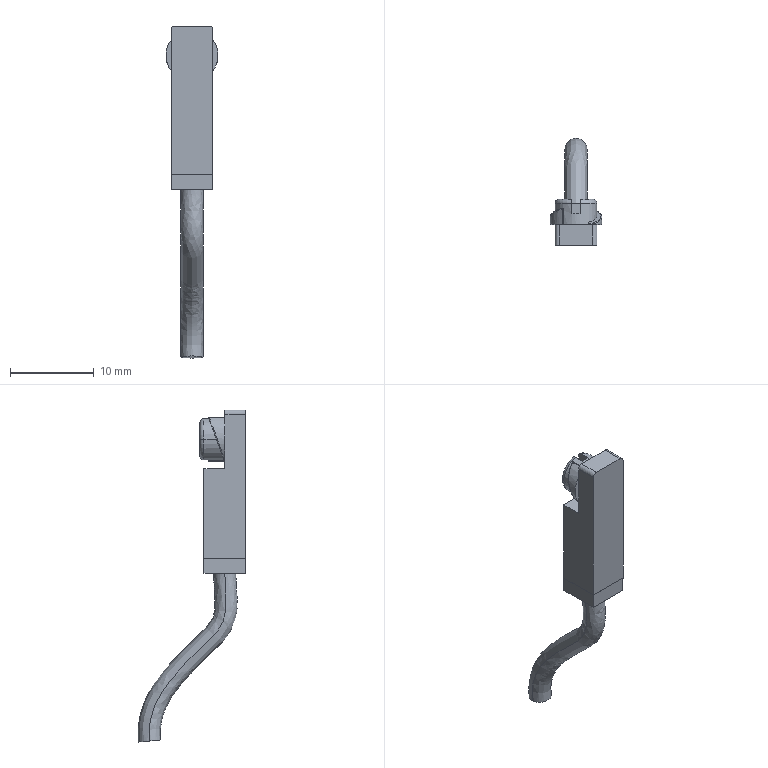Part | STEP file | Magnetic sensor switch DGN | 1 solid | 63 faces | box 6.2 x 12.865 x 39.622 mm | volume 580.439 mm3 | plane 39 | cylinder 15 | spline 4 | torus 3 | sphere 2 | commonest cylinder face diameters 0.2 x4 0.6 x4 6.2 x3 1 x2 5 x2